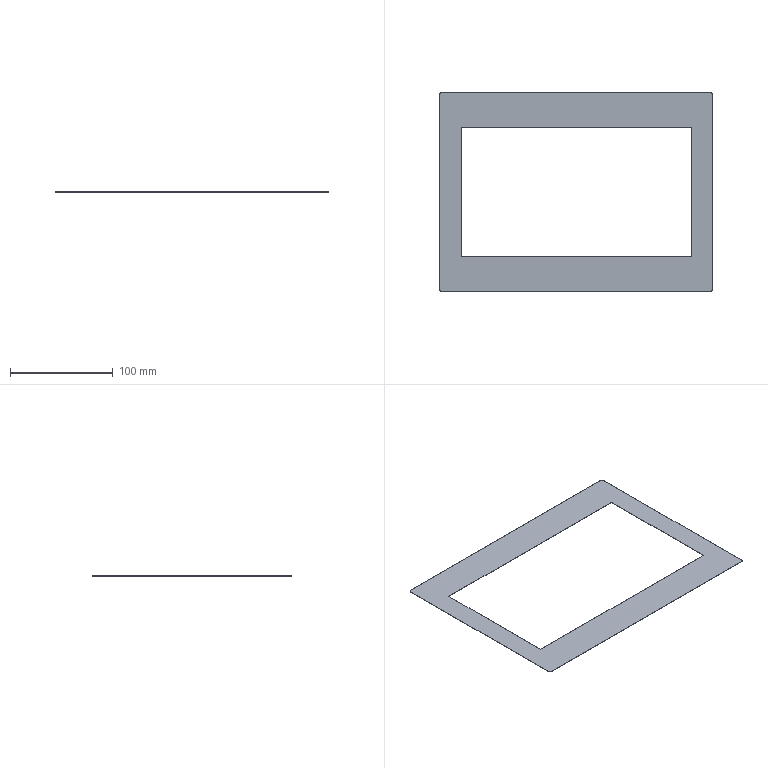Part | SolidWorks | features BaseBody 1 | 1 solid | 14 faces | box 265 x 193 x 0.32 mm | volume 7343 mm3 | plane 10 | cylinder 4 | commonest cylinder face diameters 3.5 x4
STEP:
#1=CARTESIAN_POINT('',(-111.6,-63.05,0.));
#2=VERTEX_POINT('',#1);
#3=CARTESIAN_POINT('',(-111.6,63.05,0.));
#4=VERTEX_POINT('',#3);
#5=CARTESIAN_POINT('',(-111.6,0.,0.));
#6=DIRECTION('',(0.,1.,0.));
#7=VECTOR('',#6,1000.);
#8=LINE('',#5,#7);
#9=EDGE_CURVE('',#2,#4,#8,.T.);
#10=ORIENTED_EDGE('',*,*,#9,.T.);
#11=CARTESIAN_POINT('',(112.,63.05,0.));
#12=VERTEX_POINT('',#11);
#13=CARTESIAN_POINT('',(0.,63.05,0.));
#14=DIRECTION('',(1.,0.,0.));
#15=VECTOR('',#14,1000.);
#16=LINE('',#13,#15);
#17=EDGE_CURVE('',#4,#12,#16,.T.);
#18=ORIENTED_EDGE('',*,*,#17,.T.);
#19=CARTESIAN_POINT('',(112.,-63.05,0.));
#20=VERTEX_POINT('',#19);
#21=CARTESIAN_POINT('',(112.,0.,0.));
#22=DIRECTION('',(0.,-1.,0.));
#23=VECTOR('',#22,1000.);
#24=LINE('',#21,#23);
#25=EDGE_CURVE('',#12,#20,#24,.T.);
#26=ORIENTED_EDGE('',*,*,#25,.T.);
#27=CARTESIAN_POINT('',(0.,-63.05,0.));
#28=DIRECTION('',(-1.,0.,0.));
#29=VECTOR('',#28,1000.);
#30=LINE('',#27,#29);
#31=EDGE_CURVE('',#20,#2,#30,.T.);
#32=ORIENTED_EDGE('',*,*,#31,.T.);
#33=EDGE_LOOP('',(#10,#18,#26,#32));
#34=FACE_BOUND('',#33,.T.);
#35=CARTESIAN_POINT('',(-130.75,96.5,0.));
#36=VERTEX_POINT('',#35);
#37=CARTESIAN_POINT('',(-132.5,94.75,0.));
#38=VERTEX_POINT('',#37);
#39=CARTESIAN_POINT('',(-130.75,94.75,0.));
#40=DIRECTION('',(0.,0.,1.));
#41=DIRECTION('',(1.,0.,0.));
#42=AXIS2_PLACEMENT_3D('',#39,#40,#41);
#43=CIRCLE('',#42,1.75);
#44=EDGE_CURVE('',#36,#38,#43,.T.);
#45=ORIENTED_EDGE('',*,*,#44,.T.);
#46=CARTESIAN_POINT('',(-132.5,-94.75,0.));
#47=VERTEX_POINT('',#46);
#48=CARTESIAN_POINT('',(-132.5,0.,0.));
#49=DIRECTION('',(0.,-1.,0.));
#50=VECTOR('',#49,1000.);
#51=LINE('',#48,#50);
#52=EDGE_CURVE('',#38,#47,#51,.T.);
#53=ORIENTED_EDGE('',*,*,#52,.T.);
#54=CARTESIAN_POINT('',(-130.75,-96.5,0.));
#55=VERTEX_POINT('',#54);
#56=CARTESIAN_POINT('',(-130.75,-94.75,0.));
#57=DIRECTION('',(0.,0.,1.));
#58=DIRECTION('',(1.,0.,0.));
#59=AXIS2_PLACEMENT_3D('',#56,#57,#58);
#60=CIRCLE('',#59,1.75);
#61=EDGE_CURVE('',#47,#55,#60,.T.);
#62=ORIENTED_EDGE('',*,*,#61,.T.);
#63=CARTESIAN_POINT('',(130.75,-96.5,0.));
#64=VERTEX_POINT('',#63);
#65=CARTESIAN_POINT('',(0.,-96.5,0.));
#66=DIRECTION('',(1.,0.,0.));
#67=VECTOR('',#66,1000.);
#68=LINE('',#65,#67);
#69=EDGE_CURVE('',#55,#64,#68,.T.);
#70=ORIENTED_EDGE('',*,*,#69,.T.);
#71=CARTESIAN_POINT('',(132.5,-94.75,0.));
#72=VERTEX_POINT('',#71);
#73=CARTESIAN_POINT('',(130.75,-94.75,0.));
#74=DIRECTION('',(0.,0.,1.));
#75=DIRECTION('',(1.,0.,0.));
#76=AXIS2_PLACEMENT_3D('',#73,#74,#75);
#77=CIRCLE('',#76,1.75);
#78=EDGE_CURVE('',#64,#72,#77,.T.);
#79=ORIENTED_EDGE('',*,*,#78,.T.);
#80=CARTESIAN_POINT('',(132.5,94.75,0.));
#81=VERTEX_POINT('',#80);
#82=CARTESIAN_POINT('',(132.5,0.,0.));
#83=DIRECTION('',(0.,1.,0.));
#84=VECTOR('',#83,1000.);
#85=LINE('',#82,#84);
#86=EDGE_CURVE('',#72,#81,#85,.T.);
#87=ORIENTED_EDGE('',*,*,#86,.T.);
#88=CARTESIAN_POINT('',(130.75,96.5,0.));
#89=VERTEX_POINT('',#88);
#90=CARTESIAN_POINT('',(130.75,94.75,0.));
#91=DIRECTION('',(0.,0.,1.));
#92=DIRECTION('',(1.,0.,0.));
#93=AXIS2_PLACEMENT_3D('',#90,#91,#92);
#94=CIRCLE('',#93,1.75);
#95=EDGE_CURVE('',#81,#89,#94,.T.);
#96=ORIENTED_EDGE('',*,*,#95,.T.);
#97=CARTESIAN_POINT('',(0.,96.5,0.));
#98=DIRECTION('',(-1.,0.,0.));
#99=VECTOR('',#98,1000.);
#100=LINE('',#97,#99);
#101=EDGE_CURVE('',#89,#36,#100,.T.);
#102=ORIENTED_EDGE('',*,*,#101,.T.);
#103=EDGE_LOOP('',(#45,#53,#62,#70,#79,#87,#96,#102));
#104=FACE_OUTER_BOUND('',#103,.T.);
#105=CARTESIAN_POINT('',(0.,0.,0.));
#106=DIRECTION('',(0.,0.,1.));
#107=DIRECTION('',(1.,0.,0.));
#108=AXIS2_PLACEMENT_3D('',#105,#106,#107);
#109=PLANE('',#108);
#110=ADVANCED_FACE('',(#34,#104),#109,.T.);
#111=CARTESIAN_POINT('',(112.,63.05,-0.32));
#112=VERTEX_POINT('',#111);
#113=CARTESIAN_POINT('',(112.,63.05,0.));
#114=DIRECTION('',(0.,0.,1.));
#115=VECTOR('',#114,1000.);
#116=LINE('',#113,#115);
#117=EDGE_CURVE('',#112,#12,#116,.T.);
#118=ORIENTED_EDGE('',*,*,#117,.T.);
#119=ORIENTED_EDGE('',*,*,#17,.F.);
#120=CARTESIAN_POINT('',(-111.6,63.05,-0.32));
#121=VERTEX_POINT('',#120);
#122=CARTESIAN_POINT('',(-111.6,63.05,0.));
#123=DIRECTION('',(0.,0.,-1.));
#124=VECTOR('',#123,1000.);
#125=LINE('',#122,#124);
#126=EDGE_CURVE('',#4,#121,#125,.T.);
#127=ORIENTED_EDGE('',*,*,#126,.T.);
#128=CARTESIAN_POINT('',(-111.6,63.05,-0.32));
#129=DIRECTION('',(1.,0.,0.));
#130=VECTOR('',#129,1000.);
#131=LINE('',#128,#130);
#132=EDGE_CURVE('',#121,#112,#131,.T.);
#133=ORIENTED_EDGE('',*,*,#132,.T.);
#134=EDGE_LOOP('',(#118,#119,#127,#133));
#135=FACE_OUTER_BOUND('',#134,.T.);
#136=CARTESIAN_POINT('',(-111.6,63.05,0.));
#137=DIRECTION('',(0.,-1.,0.));
#138=DIRECTION('',(0.,0.,-1.));
#139=AXIS2_PLACEMENT_3D('',#136,#137,#138);
#140=PLANE('',#139);
#141=ADVANCED_FACE('',(#135),#140,.T.);
#142=ORIENTED_EDGE('',*,*,#126,.F.);
#143=ORIENTED_EDGE('',*,*,#9,.F.);
#144=CARTESIAN_POINT('',(-111.6,-63.05,-0.32));
#145=VERTEX_POINT('',#144);
#146=CARTESIAN_POINT('',(-111.6,-63.05,0.));
#147=DIRECTION('',(0.,0.,-1.));
#148=VECTOR('',#147,1000.);
#149=LINE('',#146,#148);
#150=EDGE_CURVE('',#2,#145,#149,.T.);
#151=ORIENTED_EDGE('',*,*,#150,.T.);
#152=CARTESIAN_POINT('',(-111.6,-63.05,-0.32));
#153=DIRECTION('',(0.,1.,0.));
#154=VECTOR('',#153,1000.);
#155=LINE('',#152,#154);
#156=EDGE_CURVE('',#145,#121,#155,.T.);
#157=ORIENTED_EDGE('',*,*,#156,.T.);
#158=EDGE_LOOP('',(#142,#143,#151,#157));
#159=FACE_OUTER_BOUND('',#158,.T.);
#160=CARTESIAN_POINT('',(-111.6,-63.05,0.));
#161=DIRECTION('',(1.,0.,0.));
#162=DIRECTION('',(0.,0.,-1.));
#163=AXIS2_PLACEMENT_3D('',#160,#161,#162);
#164=PLANE('',#163);
#165=ADVANCED_FACE('',(#159),#164,.T.);
#166=ORIENTED_EDGE('',*,*,#150,.F.);
#167=ORIENTED_EDGE('',*,*,#31,.F.);
#168=CARTESIAN_POINT('',(112.,-63.05,-0.32));
#169=VERTEX_POINT('',#168);
#170=CARTESIAN_POINT('',(112.,-63.05,0.));
#171=DIRECTION('',(0.,0.,-1.));
#172=VECTOR('',#171,1000.);
#173=LINE('',#170,#172);
#174=EDGE_CURVE('',#20,#169,#173,.T.);
#175=ORIENTED_EDGE('',*,*,#174,.T.);
#176=CARTESIAN_POINT('',(112.,-63.05,-0.32));
#177=DIRECTION('',(-1.,0.,0.));
#178=VECTOR('',#177,1000.);
#179=LINE('',#176,#178);
#180=EDGE_CURVE('',#169,#145,#179,.T.);
#181=ORIENTED_EDGE('',*,*,#180,.T.);
#182=EDGE_LOOP('',(#166,#167,#175,#181));
#183=FACE_OUTER_BOUND('',#182,.T.);
#184=CARTESIAN_POINT('',(112.,-63.05,0.));
#185=DIRECTION('',(0.,1.,0.));
#186=DIRECTION('',(0.,0.,1.));
#187=AXIS2_PLACEMENT_3D('',#184,#185,#186);
#188=PLANE('',#187);
#189=ADVANCED_FACE('',(#183),#188,.T.);
#190=ORIENTED_EDGE('',*,*,#174,.F.);
#191=ORIENTED_EDGE('',*,*,#25,.F.);
#192=ORIENTED_EDGE('',*,*,#117,.F.);
#193=CARTESIAN_POINT('',(112.,63.05,-0.32));
#194=DIRECTION('',(0.,-1.,0.));
#195=VECTOR('',#194,1000.);
#196=LINE('',#193,#195);
#197=EDGE_CURVE('',#112,#169,#196,.T.);
#198=ORIENTED_EDGE('',*,*,#197,.T.);
#199=EDGE_LOOP('',(#190,#191,#192,#198));
#200=FACE_OUTER_BOUND('',#199,.T.);
#201=CARTESIAN_POINT('',(112.,63.05,0.));
#202=DIRECTION('',(-1.,0.,0.));
#203=DIRECTION('',(0.,0.,1.));
#204=AXIS2_PLACEMENT_3D('',#201,#202,#203);
#205=PLANE('',#204);
#206=ADVANCED_FACE('',(#200),#205,.T.);
#207=CARTESIAN_POINT('',(-132.5,-94.75,-0.32));
#208=VERTEX_POINT('',#207);
#209=CARTESIAN_POINT('',(-132.5,-94.75,0.));
#210=DIRECTION('',(0.,0.,1.));
#211=VECTOR('',#210,1000.);
#212=LINE('',#209,#211);
#213=EDGE_CURVE('',#208,#47,#212,.T.);
#214=ORIENTED_EDGE('',*,*,#213,.T.);
#215=ORIENTED_EDGE('',*,*,#52,.F.);
#216=CARTESIAN_POINT('',(-132.5,94.75,-0.32));
#217=VERTEX_POINT('',#216);
#218=CARTESIAN_POINT('',(-132.5,94.75,0.));
#219=DIRECTION('',(0.,0.,-1.));
#220=VECTOR('',#219,1000.);
#221=LINE('',#218,#220);
#222=EDGE_CURVE('',#38,#217,#221,.T.);
#223=ORIENTED_EDGE('',*,*,#222,.T.);
#224=CARTESIAN_POINT('',(-132.5,94.75,-0.32));
#225=DIRECTION('',(0.,-1.,0.));
#226=VECTOR('',#225,1000.);
#227=LINE('',#224,#226);
#228=EDGE_CURVE('',#217,#208,#227,.T.);
#229=ORIENTED_EDGE('',*,*,#228,.T.);
#230=EDGE_LOOP('',(#214,#215,#223,#229));
#231=FACE_OUTER_BOUND('',#230,.T.);
#232=CARTESIAN_POINT('',(-132.5,94.75,0.));
#233=DIRECTION('',(-1.,0.,0.));
#234=DIRECTION('',(0.,0.,1.));
#235=AXIS2_PLACEMENT_3D('',#232,#233,#234);
#236=PLANE('',#235);
#237=ADVANCED_FACE('',(#231),#236,.T.);
#238=ORIENTED_EDGE('',*,*,#222,.F.);
#239=ORIENTED_EDGE('',*,*,#44,.F.);
#240=CARTESIAN_POINT('',(-130.75,96.5,-0.32));
#241=VERTEX_POINT('',#240);
#242=CARTESIAN_POINT('',(-130.75,96.5,0.));
#243=DIRECTION('',(0.,0.,-1.));
#244=VECTOR('',#243,1000.);
#245=LINE('',#242,#244);
#246=EDGE_CURVE('',#36,#241,#245,.T.);
#247=ORIENTED_EDGE('',*,*,#246,.T.);
#248=CARTESIAN_POINT('',(-130.75,94.75,-0.32));
#249=DIRECTION('',(0.,0.,1.));
#250=DIRECTION('',(1.,0.,0.));
#251=AXIS2_PLACEMENT_3D('',#248,#249,#250);
#252=CIRCLE('',#251,1.75);
#253=EDGE_CURVE('',#241,#217,#252,.T.);
#254=ORIENTED_EDGE('',*,*,#253,.T.);
#255=EDGE_LOOP('',(#238,#239,#247,#254));
#256=FACE_OUTER_BOUND('',#255,.T.);
#257=CARTESIAN_POINT('',(-130.75,94.75,0.));
#258=DIRECTION('',(0.,0.,1.));
#259=DIRECTION('',(1.,0.,0.));
#260=AXIS2_PLACEMENT_3D('',#257,#258,#259);
#261=CYLINDRICAL_SURFACE('',#260,1.75);
#262=ADVANCED_FACE('',(#256),#261,.T.);
#263=ORIENTED_EDGE('',*,*,#246,.F.);
#264=ORIENTED_EDGE('',*,*,#101,.F.);
#265=CARTESIAN_POINT('',(130.75,96.5,-0.32));
#266=VERTEX_POINT('',#265);
#267=CARTESIAN_POINT('',(130.75,96.5,0.));
#268=DIRECTION('',(0.,0.,-1.));
#269=VECTOR('',#268,1000.);
#270=LINE('',#267,#269);
#271=EDGE_CURVE('',#89,#266,#270,.T.);
#272=ORIENTED_EDGE('',*,*,#271,.T.);
#273=CARTESIAN_POINT('',(130.75,96.5,-0.32));
#274=DIRECTION('',(-1.,0.,0.));
#275=VECTOR('',#274,1000.);
#276=LINE('',#273,#275);
#277=EDGE_CURVE('',#266,#241,#276,.T.);
#278=ORIENTED_EDGE('',*,*,#277,.T.);
#279=EDGE_LOOP('',(#263,#264,#272,#278));
#280=FACE_OUTER_BOUND('',#279,.T.);
#281=CARTESIAN_POINT('',(130.75,96.5,0.));
#282=DIRECTION('',(0.,1.,0.));
#283=DIRECTION('',(0.,0.,1.));
#284=AXIS2_PLACEMENT_3D('',#281,#282,#283);
#285=PLANE('',#284);
#286=ADVANCED_FACE('',(#280),#285,.T.);
#287=ORIENTED_EDGE('',*,*,#271,.F.);
#288=ORIENTED_EDGE('',*,*,#95,.F.);
#289=CARTESIAN_POINT('',(132.5,94.75,-0.32));
#290=VERTEX_POINT('',#289);
#291=CARTESIAN_POINT('',(132.5,94.75,0.));
#292=DIRECTION('',(0.,0.,-1.));
#293=VECTOR('',#292,1000.);
#294=LINE('',#291,#293);
#295=EDGE_CURVE('',#81,#290,#294,.T.);
#296=ORIENTED_EDGE('',*,*,#295,.T.);
#297=CARTESIAN_POINT('',(130.75,94.75,-0.32));
#298=DIRECTION('',(0.,0.,1.));
#299=DIRECTION('',(1.,0.,0.));
#300=AXIS2_PLACEMENT_3D('',#297,#298,#299);
#301=CIRCLE('',#300,1.75);
#302=EDGE_CURVE('',#290,#266,#301,.T.);
#303=ORIENTED_EDGE('',*,*,#302,.T.);
#304=EDGE_LOOP('',(#287,#288,#296,#303));
#305=FACE_OUTER_BOUND('',#304,.T.);
#306=CARTESIAN_POINT('',(130.75,94.75,0.));
#307=DIRECTION('',(0.,0.,1.));
#308=DIRECTION('',(1.,0.,0.));
#309=AXIS2_PLACEMENT_3D('',#306,#307,#308);
#310=CYLINDRICAL_SURFACE('',#309,1.75);
#311=ADVANCED_FACE('',(#305),#310,.T.);
#312=ORIENTED_EDGE('',*,*,#295,.F.);
#313=ORIENTED_EDGE('',*,*,#86,.F.);
#314=CARTESIAN_POINT('',(132.5,-94.75,-0.32));
#315=VERTEX_POINT('',#314);
#316=CARTESIAN_POINT('',(132.5,-94.75,0.));
#317=DIRECTION('',(0.,0.,-1.));
#318=VECTOR('',#317,1000.);
#319=LINE('',#316,#318);
#320=EDGE_CURVE('',#72,#315,#319,.T.);
#321=ORIENTED_EDGE('',*,*,#320,.T.);
#322=CARTESIAN_POINT('',(132.5,-94.75,-0.32));
#323=DIRECTION('',(0.,1.,0.));
#324=VECTOR('',#323,1000.);
#325=LINE('',#322,#324);
#326=EDGE_CURVE('',#315,#290,#325,.T.);
#327=ORIENTED_EDGE('',*,*,#326,.T.);
#328=EDGE_LOOP('',(#312,#313,#321,#327));
#329=FACE_OUTER_BOUND('',#328,.T.);
#330=CARTESIAN_POINT('',(132.5,-94.75,0.));
#331=DIRECTION('',(1.,0.,0.));
#332=DIRECTION('',(0.,0.,-1.));
#333=AXIS2_PLACEMENT_3D('',#330,#331,#332);
#334=PLANE('',#333);
#335=ADVANCED_FACE('',(#329),#334,.T.);
#336=ORIENTED_EDGE('',*,*,#320,.F.);
#337=ORIENTED_EDGE('',*,*,#78,.F.);
#338=CARTESIAN_POINT('',(130.75,-96.5,-0.32));
#339=VERTEX_POINT('',#338);
#340=CARTESIAN_POINT('',(130.75,-96.5,0.));
#341=DIRECTION('',(0.,0.,-1.));
#342=VECTOR('',#341,1000.);
#343=LINE('',#340,#342);
#344=EDGE_CURVE('',#64,#339,#343,.T.);
#345=ORIENTED_EDGE('',*,*,#344,.T.);
#346=CARTESIAN_POINT('',(130.75,-94.75,-0.32));
#347=DIRECTION('',(0.,0.,1.));
#348=DIRECTION('',(1.,0.,0.));
#349=AXIS2_PLACEMENT_3D('',#346,#347,#348);
#350=CIRCLE('',#349,1.75);
#351=EDGE_CURVE('',#339,#315,#350,.T.);
#352=ORIENTED_EDGE('',*,*,#351,.T.);
#353=EDGE_LOOP('',(#336,#337,#345,#352));
#354=FACE_OUTER_BOUND('',#353,.T.);
#355=CARTESIAN_POINT('',(130.75,-94.75,0.));
#356=DIRECTION('',(0.,0.,1.));
#357=DIRECTION('',(1.,0.,0.));
#358=AXIS2_PLACEMENT_3D('',#355,#356,#357);
#359=CYLINDRICAL_SURFACE('',#358,1.75);
#360=ADVANCED_FACE('',(#354),#359,.T.);
#361=ORIENTED_EDGE('',*,*,#344,.F.);
#362=ORIENTED_EDGE('',*,*,#69,.F.);
#363=CARTESIAN_POINT('',(-130.75,-96.5,-0.32));
#364=VERTEX_POINT('',#363);
#365=CARTESIAN_POINT('',(-130.75,-96.5,0.));
#366=DIRECTION('',(0.,0.,-1.));
#367=VECTOR('',#366,1000.);
#368=LINE('',#365,#367);
#369=EDGE_CURVE('',#55,#364,#368,.T.);
#370=ORIENTED_EDGE('',*,*,#369,.T.);
#371=CARTESIAN_POINT('',(-130.75,-96.5,-0.32));
#372=DIRECTION('',(1.,0.,0.));
#373=VECTOR('',#372,1000.);
#374=LINE('',#371,#373);
#375=EDGE_CURVE('',#364,#339,#374,.T.);
#376=ORIENTED_EDGE('',*,*,#375,.T.);
#377=EDGE_LOOP('',(#361,#362,#370,#376));
#378=FACE_OUTER_BOUND('',#377,.T.);
#379=CARTESIAN_POINT('',(-130.75,-96.5,0.));
#380=DIRECTION('',(0.,-1.,0.));
#381=DIRECTION('',(0.,0.,-1.));
#382=AXIS2_PLACEMENT_3D('',#379,#380,#381);
#383=PLANE('',#382);
#384=ADVANCED_FACE('',(#378),#383,.T.);
#385=ORIENTED_EDGE('',*,*,#369,.F.);
#386=ORIENTED_EDGE('',*,*,#61,.F.);
#387=ORIENTED_EDGE('',*,*,#213,.F.);
#388=CARTESIAN_POINT('',(-130.75,-94.75,-0.32));
#389=DIRECTION('',(0.,0.,1.));
#390=DIRECTION('',(1.,0.,0.));
#391=AXIS2_PLACEMENT_3D('',#388,#389,#390);
#392=CIRCLE('',#391,1.75);
#393=EDGE_CURVE('',#208,#364,#392,.T.);
#394=ORIENTED_EDGE('',*,*,#393,.T.);
#395=EDGE_LOOP('',(#385,#386,#387,#394));
#396=FACE_OUTER_BOUND('',#395,.T.);
#397=CARTESIAN_POINT('',(-130.75,-94.75,0.));
#398=DIRECTION('',(0.,0.,1.));
#399=DIRECTION('',(1.,0.,0.));
#400=AXIS2_PLACEMENT_3D('',#397,#398,#399);
#401=CYLINDRICAL_SURFACE('',#400,1.75);
#402=ADVANCED_FACE('',(#396),#401,.T.);
#403=ORIENTED_EDGE('',*,*,#180,.F.);
#404=ORIENTED_EDGE('',*,*,#197,.F.);
#405=ORIENTED_EDGE('',*,*,#132,.F.);
#406=ORIENTED_EDGE('',*,*,#156,.F.);
#407=EDGE_LOOP('',(#403,#404,#405,#406));
#408=FACE_BOUND('',#407,.T.);
#409=ORIENTED_EDGE('',*,*,#277,.F.);
#410=ORIENTED_EDGE('',*,*,#302,.F.);
#411=ORIENTED_EDGE('',*,*,#326,.F.);
#412=ORIENTED_EDGE('',*,*,#351,.F.);
#413=ORIENTED_EDGE('',*,*,#375,.F.);
#414=ORIENTED_EDGE('',*,*,#393,.F.);
#415=ORIENTED_EDGE('',*,*,#228,.F.);
#416=ORIENTED_EDGE('',*,*,#253,.F.);
#417=EDGE_LOOP('',(#409,#410,#411,#412,#413,#414,#415,#416));
#418=FACE_OUTER_BOUND('',#417,.T.);
#419=CARTESIAN_POINT('',(0.,0.,-0.32));
#420=DIRECTION('',(0.,0.,1.));
#421=DIRECTION('',(1.,0.,0.));
#422=AXIS2_PLACEMENT_3D('',#419,#420,#421);
#423=PLANE('',#422);
#424=ADVANCED_FACE('',(#408,#418),#423,.F.);
#425=CLOSED_SHELL('',(#110,#141,#165,#189,#206,#237,#262,#286,#311,#335,#360,#384,#402,#424));
#426=MANIFOLD_SOLID_BREP('',#425);
#427=CARTESIAN_POINT('',(0.,0.,0.));
#428=DIRECTION('',(0.,0.,1.));
#429=DIRECTION('',(1.,0.,0.));
#430=AXIS2_PLACEMENT_3D('',#427,#428,#429);
#431=(LENGTH_UNIT()NAMED_UNIT(*)SI_UNIT(.MILLI.,.METRE.));
#432=UNCERTAINTY_MEASURE_WITH_UNIT(LENGTH_MEASURE(0.00001),#431,'','');
#433=(NAMED_UNIT(*)PLANE_ANGLE_UNIT()SI_UNIT($,.RADIAN.));
#434=(NAMED_UNIT(*)SI_UNIT($,.STERADIAN.)SOLID_ANGLE_UNIT());
#435=(GEOMETRIC_REPRESENTATION_CONTEXT(3)GLOBAL_UNCERTAINTY_ASSIGNED_CONTEXT((#432))GLOBAL_UNIT_ASSIGNED_CONTEXT((#431,#433,#434))REPRESENTATION_CONTEXT('',''));
#436=ADVANCED_BREP_SHAPE_REPRESENTATION('',(#426,#430),#435);